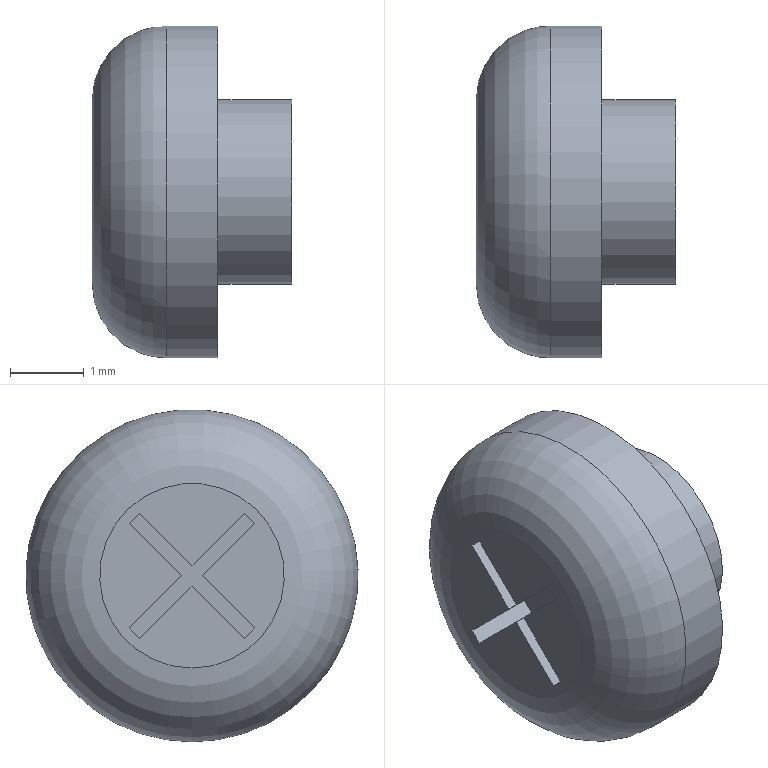Part | STEP file | 1 solid | 19 faces | box 2.7 x 4.5 x 4.5 mm | volume 28.373 mm3 | plane 16 | cylinder 2 | torus 1 | commonest cylinder face diameters 2.5 x1 4.5 x1
STEP:
#1=CARTESIAN_POINT('',(0.,0.,0.));
#2=DIRECTION('',(0.,0.,1.));
#3=DIRECTION('',(1.,0.,0.));
#4=AXIS2_PLACEMENT_3D('',#1,#2,#3);
#5=CARTESIAN_POINT('',(0.,0.,-1.25));
#6=VERTEX_POINT('',#5);
#7=CARTESIAN_POINT('',(0.,0.,0.));
#8=DIRECTION('',(-1.,0.,0.));
#9=DIRECTION('',(0.,0.,-1.));
#10=AXIS2_PLACEMENT_3D('',#7,#8,#9);
#11=CIRCLE('',#10,1.25);
#12=CARTESIAN_POINT('',(0.,0.,0.));
#13=DIRECTION('',(1.,0.,0.));
#14=DIRECTION('',(0.,0.,-1.));
#15=AXIS2_PLACEMENT_3D('',#12,#13,#14);
#16=PLANE('',#15);
#17=CARTESIAN_POINT('',(1.25,0.));
#18=CARTESIAN_POINT('',(1.25,-2.165));
#19=CARTESIAN_POINT('',(-0.625,-1.083));
#20=CARTESIAN_POINT('',(-2.5,0.));
#21=CARTESIAN_POINT('',(-0.625,1.083));
#22=CARTESIAN_POINT('',(1.25,2.165));
#23=CARTESIAN_POINT('',(1.25,0.));
#24=(BOUNDED_CURVE()B_SPLINE_CURVE(2,(#17,#18,#19,#20,#21,#22,#23),.UNSPECIFIED.,.T.,.F.)B_SPLINE_CURVE_WITH_KNOTS((1,2,2,2,2,1),(-2.094,0.,2.094,4.189,6.283,8.378),.UNSPECIFIED.)CURVE()GEOMETRIC_REPRESENTATION_ITEM()RATIONAL_B_SPLINE_CURVE((1.,0.5,1.,0.5,1.,0.5,1.))REPRESENTATION_ITEM(''));
#25=(GEOMETRIC_REPRESENTATION_CONTEXT(2)PARAMETRIC_REPRESENTATION_CONTEXT()REPRESENTATION_CONTEXT('',''));
#26=DEFINITIONAL_REPRESENTATION('',(#24),#25);
#27=PCURVE('',#16,#26);
#28=CARTESIAN_POINT('',(-1.835,0.,0.));
#29=DIRECTION('',(1.,0.,0.));
#30=DIRECTION('',(0.,0.,-1.));
#31=AXIS2_PLACEMENT_3D('',#28,#29,#30);
#32=CYLINDRICAL_SURFACE('',#31,1.25);
#33=CARTESIAN_POINT('',(6.283,1.835));
#34=DIRECTION('',(-1.,0.));
#35=VECTOR('',#34,1.);
#36=LINE('',#33,#35);
#37=(GEOMETRIC_REPRESENTATION_CONTEXT(2)PARAMETRIC_REPRESENTATION_CONTEXT()REPRESENTATION_CONTEXT('',''));
#38=DEFINITIONAL_REPRESENTATION('',(#36),#37);
#39=PCURVE('',#32,#38);
#40=SURFACE_CURVE('',#11,(#27,#39),.PCURVE_S1.);
#41=EDGE_CURVE('',#6,#6,#40,.T.);
#42=ORIENTED_EDGE('',*,*,#41,.T.);
#43=EDGE_LOOP('',(#42));
#44=FACE_BOUND('',#43,.T.);
#45=CARTESIAN_POINT('',(0.,0.,-2.25));
#46=VERTEX_POINT('',#45);
#47=CARTESIAN_POINT('',(0.,0.,0.));
#48=DIRECTION('',(1.,0.,0.));
#49=DIRECTION('',(0.,0.,-1.));
#50=AXIS2_PLACEMENT_3D('',#47,#48,#49);
#51=CIRCLE('',#50,2.25);
#52=CARTESIAN_POINT('',(0.,0.));
#53=DIRECTION('',(1.,0.));
#54=AXIS2_PLACEMENT_2D('',#52,#53);
#55=CIRCLE('',#54,2.25);
#56=(GEOMETRIC_REPRESENTATION_CONTEXT(2)PARAMETRIC_REPRESENTATION_CONTEXT()REPRESENTATION_CONTEXT('',''));
#57=DEFINITIONAL_REPRESENTATION('',(#55),#56);
#58=PCURVE('',#16,#57);
#59=CARTESIAN_POINT('',(-1.835,0.,0.));
#60=DIRECTION('',(1.,0.,0.));
#61=DIRECTION('',(0.,0.,-1.));
#62=AXIS2_PLACEMENT_3D('',#59,#60,#61);
#63=CYLINDRICAL_SURFACE('',#62,2.25);
#64=CARTESIAN_POINT('',(0.,1.835));
#65=DIRECTION('',(1.,0.));
#66=VECTOR('',#65,1.);
#67=LINE('',#64,#66);
#68=(GEOMETRIC_REPRESENTATION_CONTEXT(2)PARAMETRIC_REPRESENTATION_CONTEXT()REPRESENTATION_CONTEXT('',''));
#69=DEFINITIONAL_REPRESENTATION('',(#67),#68);
#70=PCURVE('',#63,#69);
#71=SURFACE_CURVE('',#51,(#58,#70),.PCURVE_S1.);
#72=EDGE_CURVE('',#46,#46,#71,.T.);
#73=ORIENTED_EDGE('',*,*,#72,.T.);
#74=EDGE_LOOP('',(#73));
#75=FACE_BOUND('',#74,.T.);
#76=ADVANCED_FACE('',(#44,#75),#16,.T.);
#77=CARTESIAN_POINT('',(1.,0.,-1.25));
#78=VERTEX_POINT('',#77);
#79=CARTESIAN_POINT('',(1.,0.,0.));
#80=DIRECTION('',(-1.,0.,0.));
#81=DIRECTION('',(0.,0.,-1.));
#82=AXIS2_PLACEMENT_3D('',#79,#80,#81);
#83=CIRCLE('',#82,1.25);
#84=CARTESIAN_POINT('',(6.283,2.835));
#85=DIRECTION('',(-1.,0.));
#86=VECTOR('',#85,1.);
#87=LINE('',#84,#86);
#88=(GEOMETRIC_REPRESENTATION_CONTEXT(2)PARAMETRIC_REPRESENTATION_CONTEXT()REPRESENTATION_CONTEXT('',''));
#89=DEFINITIONAL_REPRESENTATION('',(#87),#88);
#90=PCURVE('',#32,#89);
#91=CARTESIAN_POINT('',(1.,0.,0.));
#92=DIRECTION('',(1.,0.,0.));
#93=DIRECTION('',(0.,0.,-1.));
#94=AXIS2_PLACEMENT_3D('',#91,#92,#93);
#95=PLANE('',#94);
#96=CARTESIAN_POINT('',(1.25,0.));
#97=CARTESIAN_POINT('',(1.25,-2.165));
#98=CARTESIAN_POINT('',(-0.625,-1.083));
#99=CARTESIAN_POINT('',(-2.5,0.));
#100=CARTESIAN_POINT('',(-0.625,1.083));
#101=CARTESIAN_POINT('',(1.25,2.165));
#102=CARTESIAN_POINT('',(1.25,0.));
#103=(BOUNDED_CURVE()B_SPLINE_CURVE(2,(#96,#97,#98,#99,#100,#101,#102),.UNSPECIFIED.,.T.,.F.)B_SPLINE_CURVE_WITH_KNOTS((1,2,2,2,2,1),(-2.094,0.,2.094,4.189,6.283,8.378),.UNSPECIFIED.)CURVE()GEOMETRIC_REPRESENTATION_ITEM()RATIONAL_B_SPLINE_CURVE((1.,0.5,1.,0.5,1.,0.5,1.))REPRESENTATION_ITEM(''));
#104=(GEOMETRIC_REPRESENTATION_CONTEXT(2)PARAMETRIC_REPRESENTATION_CONTEXT()REPRESENTATION_CONTEXT('',''));
#105=DEFINITIONAL_REPRESENTATION('',(#103),#104);
#106=PCURVE('',#95,#105);
#107=SURFACE_CURVE('',#83,(#90,#106),.PCURVE_S1.);
#108=EDGE_CURVE('',#78,#78,#107,.T.);
#109=ORIENTED_EDGE('',*,*,#108,.T.);
#110=CARTESIAN_POINT('',(0.,0.,-1.25));
#111=CARTESIAN_POINT('',(1.,0.,-1.25));
#112=B_SPLINE_CURVE_WITH_KNOTS('',1,(#110,#111),.UNSPECIFIED.,.F.,.F.,(2,2),(1.835,2.835),.PIECEWISE_BEZIER_KNOTS.);
#113=CARTESIAN_POINT('',(0.,0.));
#114=DIRECTION('',(0.,1.));
#115=VECTOR('',#114,1.);
#116=LINE('',#113,#115);
#117=(GEOMETRIC_REPRESENTATION_CONTEXT(2)PARAMETRIC_REPRESENTATION_CONTEXT()REPRESENTATION_CONTEXT('',''));
#118=DEFINITIONAL_REPRESENTATION('',(#116),#117);
#119=PCURVE('',#32,#118);
#120=CARTESIAN_POINT('',(6.283,0.));
#121=DIRECTION('',(0.,1.));
#122=VECTOR('',#121,1.);
#123=LINE('',#120,#122);
#124=(GEOMETRIC_REPRESENTATION_CONTEXT(2)PARAMETRIC_REPRESENTATION_CONTEXT()REPRESENTATION_CONTEXT('',''));
#125=DEFINITIONAL_REPRESENTATION('',(#123),#124);
#126=PCURVE('',#32,#125);
#127=SEAM_CURVE('',#112,(#119,#126),.PCURVE_S1.);
#128=EDGE_CURVE('',#6,#78,#127,.T.);
#129=ORIENTED_EDGE('',*,*,#128,.F.);
#130=ORIENTED_EDGE('',*,*,#41,.F.);
#131=ORIENTED_EDGE('',*,*,#128,.T.);
#132=EDGE_LOOP('',(#109,#129,#130,#131));
#133=FACE_BOUND('',#132,.T.);
#134=ADVANCED_FACE('',(#133),#32,.T.);
#135=CARTESIAN_POINT('',(-0.7,0.,-2.25));
#136=VERTEX_POINT('',#135);
#137=CARTESIAN_POINT('',(-0.7,0.,0.));
#138=DIRECTION('',(1.,0.,0.));
#139=DIRECTION('',(0.,0.,-1.));
#140=AXIS2_PLACEMENT_3D('',#137,#138,#139);
#141=CIRCLE('',#140,2.25);
#142=CARTESIAN_POINT('',(0.,1.135));
#143=DIRECTION('',(1.,0.));
#144=VECTOR('',#143,1.);
#145=LINE('',#142,#144);
#146=(GEOMETRIC_REPRESENTATION_CONTEXT(2)PARAMETRIC_REPRESENTATION_CONTEXT()REPRESENTATION_CONTEXT('',''));
#147=DEFINITIONAL_REPRESENTATION('',(#145),#146);
#148=PCURVE('',#63,#147);
#149=CARTESIAN_POINT('',(-0.7,0.,0.));
#150=DIRECTION('',(1.,0.,0.));
#151=DIRECTION('',(0.,0.,-1.));
#152=AXIS2_PLACEMENT_3D('',#149,#150,#151);
#153=TOROIDAL_SURFACE('',#152,1.25,1.);
#154=CARTESIAN_POINT('',(0.,6.283));
#155=DIRECTION('',(1.,0.));
#156=VECTOR('',#155,1.);
#157=LINE('',#154,#156);
#158=(GEOMETRIC_REPRESENTATION_CONTEXT(2)PARAMETRIC_REPRESENTATION_CONTEXT()REPRESENTATION_CONTEXT('',''));
#159=DEFINITIONAL_REPRESENTATION('',(#157),#158);
#160=PCURVE('',#153,#159);
#161=SURFACE_CURVE('',#141,(#148,#160),.PCURVE_S1.);
#162=EDGE_CURVE('',#136,#136,#161,.T.);
#163=ORIENTED_EDGE('',*,*,#162,.T.);
#164=CARTESIAN_POINT('',(-0.7,0.,-2.25));
#165=CARTESIAN_POINT('',(0.,0.,-2.25));
#166=B_SPLINE_CURVE_WITH_KNOTS('',1,(#164,#165),.UNSPECIFIED.,.F.,.F.,(2,2),(1.135,1.835),.PIECEWISE_BEZIER_KNOTS.);
#167=CARTESIAN_POINT('',(6.283,0.));
#168=DIRECTION('',(0.,1.));
#169=VECTOR('',#168,1.);
#170=LINE('',#167,#169);
#171=(GEOMETRIC_REPRESENTATION_CONTEXT(2)PARAMETRIC_REPRESENTATION_CONTEXT()REPRESENTATION_CONTEXT('',''));
#172=DEFINITIONAL_REPRESENTATION('',(#170),#171);
#173=PCURVE('',#63,#172);
#174=CARTESIAN_POINT('',(0.,0.));
#175=DIRECTION('',(0.,1.));
#176=VECTOR('',#175,1.);
#177=LINE('',#174,#176);
#178=(GEOMETRIC_REPRESENTATION_CONTEXT(2)PARAMETRIC_REPRESENTATION_CONTEXT()REPRESENTATION_CONTEXT('',''));
#179=DEFINITIONAL_REPRESENTATION('',(#177),#178);
#180=PCURVE('',#63,#179);
#181=SEAM_CURVE('',#166,(#173,#180),.PCURVE_S1.);
#182=EDGE_CURVE('',#136,#46,#181,.T.);
#183=ORIENTED_EDGE('',*,*,#182,.T.);
#184=ORIENTED_EDGE('',*,*,#72,.F.);
#185=ORIENTED_EDGE('',*,*,#182,.F.);
#186=EDGE_LOOP('',(#163,#183,#184,#185));
#187=FACE_BOUND('',#186,.T.);
#188=ADVANCED_FACE('',(#187),#63,.T.);
#189=ORIENTED_EDGE('',*,*,#108,.F.);
#190=EDGE_LOOP('',(#189));
#191=FACE_BOUND('',#190,.T.);
#192=ADVANCED_FACE('',(#191),#95,.T.);
#193=ORIENTED_EDGE('',*,*,#162,.F.);
#194=CARTESIAN_POINT('',(-1.7,0.,-1.25));
#195=VERTEX_POINT('',#194);
#196=CARTESIAN_POINT('',(-1.7,0.,-1.25));
#197=CARTESIAN_POINT('',(-1.7,0.,-1.517));
#198=CARTESIAN_POINT('',(-1.615,0.,-1.778));
#199=CARTESIAN_POINT('',(-1.452,0.,-2.002));
#200=CARTESIAN_POINT('',(-1.228,0.,-2.165));
#201=CARTESIAN_POINT('',(-0.9673,0.,-2.25));
#202=CARTESIAN_POINT('',(-0.7,0.,-2.25));
#203=(BOUNDED_CURVE()B_SPLINE_CURVE(6,(#196,#197,#198,#199,#200,#201,#202),.UNSPECIFIED.,.F.,.F.)B_SPLINE_CURVE_WITH_KNOTS((7,7),(4.712,6.283),.PIECEWISE_BEZIER_KNOTS.)CURVE()GEOMETRIC_REPRESENTATION_ITEM()RATIONAL_B_SPLINE_CURVE((1.031,1.01,0.9979,0.994,0.9979,1.01,1.031))REPRESENTATION_ITEM(''));
#204=CARTESIAN_POINT('',(0.,0.));
#205=DIRECTION('',(0.,1.));
#206=VECTOR('',#205,1.);
#207=LINE('',#204,#206);
#208=(GEOMETRIC_REPRESENTATION_CONTEXT(2)PARAMETRIC_REPRESENTATION_CONTEXT()REPRESENTATION_CONTEXT('',''));
#209=DEFINITIONAL_REPRESENTATION('',(#207),#208);
#210=PCURVE('',#153,#209);
#211=CARTESIAN_POINT('',(6.283,0.));
#212=DIRECTION('',(0.,1.));
#213=VECTOR('',#212,1.);
#214=LINE('',#211,#213);
#215=(GEOMETRIC_REPRESENTATION_CONTEXT(2)PARAMETRIC_REPRESENTATION_CONTEXT()REPRESENTATION_CONTEXT('',''));
#216=DEFINITIONAL_REPRESENTATION('',(#214),#215);
#217=PCURVE('',#153,#216);
#218=SEAM_CURVE('',#203,(#210,#217),.PCURVE_S1.);
#219=EDGE_CURVE('',#195,#136,#218,.T.);
#220=ORIENTED_EDGE('',*,*,#219,.F.);
#221=CARTESIAN_POINT('',(-1.7,0.,0.));
#222=DIRECTION('',(1.,0.,0.));
#223=DIRECTION('',(0.,0.,-1.));
#224=AXIS2_PLACEMENT_3D('',#221,#222,#223);
#225=CIRCLE('',#224,1.25);
#226=CARTESIAN_POINT('',(0.,4.712));
#227=DIRECTION('',(1.,0.));
#228=VECTOR('',#227,1.);
#229=LINE('',#226,#228);
#230=(GEOMETRIC_REPRESENTATION_CONTEXT(2)PARAMETRIC_REPRESENTATION_CONTEXT()REPRESENTATION_CONTEXT('',''));
#231=DEFINITIONAL_REPRESENTATION('',(#229),#230);
#232=PCURVE('',#153,#231);
#233=CARTESIAN_POINT('',(-1.7,0.,0.));
#234=DIRECTION('',(1.,0.,0.));
#235=DIRECTION('',(0.,0.,-1.));
#236=AXIS2_PLACEMENT_3D('',#233,#234,#235);
#237=PLANE('',#236);
#238=CARTESIAN_POINT('',(0.,0.));
#239=DIRECTION('',(1.,0.));
#240=AXIS2_PLACEMENT_2D('',#238,#239);
#241=CIRCLE('',#240,1.25);
#242=(GEOMETRIC_REPRESENTATION_CONTEXT(2)PARAMETRIC_REPRESENTATION_CONTEXT()REPRESENTATION_CONTEXT('',''));
#243=DEFINITIONAL_REPRESENTATION('',(#241),#242);
#244=PCURVE('',#237,#243);
#245=SURFACE_CURVE('',#225,(#232,#244),.PCURVE_S1.);
#246=EDGE_CURVE('',#195,#195,#245,.T.);
#247=ORIENTED_EDGE('',*,*,#246,.T.);
#248=ORIENTED_EDGE('',*,*,#219,.T.);
#249=EDGE_LOOP('',(#193,#220,#247,#248));
#250=FACE_BOUND('',#249,.T.);
#251=ADVANCED_FACE('',(#250),#153,.T.);
#252=CARTESIAN_POINT('',(-1.7,0.8485,0.7071));
#253=VERTEX_POINT('',#252);
#254=CARTESIAN_POINT('',(-1.7,0.1414,0.));
#255=VERTEX_POINT('',#254);
#256=CARTESIAN_POINT('',(-1.7,0.8485,0.7071));
#257=DIRECTION('',(0.,-0.7071,-0.7071));
#258=VECTOR('',#257,1.);
#259=LINE('',#256,#258);
#260=CARTESIAN_POINT('',(-0.7071,0.8485));
#261=DIRECTION('',(0.7071,-0.7071));
#262=VECTOR('',#261,1.);
#263=LINE('',#260,#262);
#264=(GEOMETRIC_REPRESENTATION_CONTEXT(2)PARAMETRIC_REPRESENTATION_CONTEXT()REPRESENTATION_CONTEXT('',''));
#265=DEFINITIONAL_REPRESENTATION('',(#263),#264);
#266=PCURVE('',#237,#265);
#267=CARTESIAN_POINT('',(-1.7,0.8485,0.7071));
#268=DIRECTION('',(0.,0.7071,-0.7071));
#269=DIRECTION('',(0.,0.7071,0.7071));
#270=AXIS2_PLACEMENT_3D('',#267,#268,#269);
#271=PLANE('',#270);
#272=CARTESIAN_POINT('',(0.,0.));
#273=DIRECTION('',(-1.,0.));
#274=VECTOR('',#273,1.);
#275=LINE('',#272,#274);
#276=(GEOMETRIC_REPRESENTATION_CONTEXT(2)PARAMETRIC_REPRESENTATION_CONTEXT()REPRESENTATION_CONTEXT('',''));
#277=DEFINITIONAL_REPRESENTATION('',(#275),#276);
#278=PCURVE('',#271,#277);
#279=SURFACE_CURVE('',#259,(#266,#278),.PCURVE_S1.);
#280=EDGE_CURVE('',#253,#255,#279,.T.);
#281=ORIENTED_EDGE('',*,*,#280,.F.);
#282=CARTESIAN_POINT('',(-1.7,0.7071,0.8485));
#283=VERTEX_POINT('',#282);
#284=CARTESIAN_POINT('',(-1.7,0.7071,0.8485));
#285=DIRECTION('',(0.,0.7071,-0.7071));
#286=VECTOR('',#285,1.);
#287=LINE('',#284,#286);
#288=CARTESIAN_POINT('',(-0.8485,0.7071));
#289=DIRECTION('',(0.7071,0.7071));
#290=VECTOR('',#289,1.);
#291=LINE('',#288,#290);
#292=(GEOMETRIC_REPRESENTATION_CONTEXT(2)PARAMETRIC_REPRESENTATION_CONTEXT()REPRESENTATION_CONTEXT('',''));
#293=DEFINITIONAL_REPRESENTATION('',(#291),#292);
#294=PCURVE('',#237,#293);
#295=CARTESIAN_POINT('',(-1.7,0.7071,0.8485));
#296=DIRECTION('',(0.,0.7071,0.7071));
#297=DIRECTION('',(0.,-0.7071,0.7071));
#298=AXIS2_PLACEMENT_3D('',#295,#296,#297);
#299=PLANE('',#298);
#300=CARTESIAN_POINT('',(0.,0.));
#301=DIRECTION('',(-1.,0.));
#302=VECTOR('',#301,1.);
#303=LINE('',#300,#302);
#304=(GEOMETRIC_REPRESENTATION_CONTEXT(2)PARAMETRIC_REPRESENTATION_CONTEXT()REPRESENTATION_CONTEXT('',''));
#305=DEFINITIONAL_REPRESENTATION('',(#303),#304);
#306=PCURVE('',#299,#305);
#307=SURFACE_CURVE('',#287,(#294,#306),.PCURVE_S1.);
#308=EDGE_CURVE('',#283,#253,#307,.T.);
#309=ORIENTED_EDGE('',*,*,#308,.F.);
#310=CARTESIAN_POINT('',(-1.7,0.,0.1414));
#311=VERTEX_POINT('',#310);
#312=CARTESIAN_POINT('',(-1.7,0.,0.1414));
#313=DIRECTION('',(0.,0.7071,0.7071));
#314=VECTOR('',#313,1.);
#315=LINE('',#312,#314);
#316=CARTESIAN_POINT('',(-0.1414,0.));
#317=DIRECTION('',(-0.7071,0.7071));
#318=VECTOR('',#317,1.);
#319=LINE('',#316,#318);
#320=(GEOMETRIC_REPRESENTATION_CONTEXT(2)PARAMETRIC_REPRESENTATION_CONTEXT()REPRESENTATION_CONTEXT('',''));
#321=DEFINITIONAL_REPRESENTATION('',(#319),#320);
#322=PCURVE('',#237,#321);
#323=CARTESIAN_POINT('',(-1.7,0.,0.1414));
#324=DIRECTION('',(0.,-0.7071,0.7071));
#325=DIRECTION('',(0.,-0.7071,-0.7071));
#326=AXIS2_PLACEMENT_3D('',#323,#324,#325);
#327=PLANE('',#326);
#328=CARTESIAN_POINT('',(0.,0.));
#329=DIRECTION('',(-1.,0.));
#330=VECTOR('',#329,1.);
#331=LINE('',#328,#330);
#332=(GEOMETRIC_REPRESENTATION_CONTEXT(2)PARAMETRIC_REPRESENTATION_CONTEXT()REPRESENTATION_CONTEXT('',''));
#333=DEFINITIONAL_REPRESENTATION('',(#331),#332);
#334=PCURVE('',#327,#333);
#335=SURFACE_CURVE('',#315,(#322,#334),.PCURVE_S1.);
#336=EDGE_CURVE('',#311,#283,#335,.T.);
#337=ORIENTED_EDGE('',*,*,#336,.F.);
#338=CARTESIAN_POINT('',(-1.7,-0.7071,0.8485));
#339=VERTEX_POINT('',#338);
#340=CARTESIAN_POINT('',(-1.7,-0.7071,0.8485));
#341=DIRECTION('',(0.,0.7071,-0.7071));
#342=VECTOR('',#341,1.);
#343=LINE('',#340,#342);
#344=CARTESIAN_POINT('',(-0.8485,-0.7071));
#345=DIRECTION('',(0.7071,0.7071));
#346=VECTOR('',#345,1.);
#347=LINE('',#344,#346);
#348=(GEOMETRIC_REPRESENTATION_CONTEXT(2)PARAMETRIC_REPRESENTATION_CONTEXT()REPRESENTATION_CONTEXT('',''));
#349=DEFINITIONAL_REPRESENTATION('',(#347),#348);
#350=PCURVE('',#237,#349);
#351=CARTESIAN_POINT('',(-1.7,-0.7071,0.8485));
#352=DIRECTION('',(0.,0.7071,0.7071));
#353=DIRECTION('',(0.,-0.7071,0.7071));
#354=AXIS2_PLACEMENT_3D('',#351,#352,#353);
#355=PLANE('',#354);
#356=CARTESIAN_POINT('',(0.,0.));
#357=DIRECTION('',(-1.,0.));
#358=VECTOR('',#357,1.);
#359=LINE('',#356,#358);
#360=(GEOMETRIC_REPRESENTATION_CONTEXT(2)PARAMETRIC_REPRESENTATION_CONTEXT()REPRESENTATION_CONTEXT('',''));
#361=DEFINITIONAL_REPRESENTATION('',(#359),#360);
#362=PCURVE('',#355,#361);
#363=SURFACE_CURVE('',#343,(#350,#362),.PCURVE_S1.);
#364=EDGE_CURVE('',#339,#311,#363,.T.);
#365=ORIENTED_EDGE('',*,*,#364,.F.);
#366=CARTESIAN_POINT('',(-1.7,-0.8485,0.7071));
#367=VERTEX_POINT('',#366);
#368=CARTESIAN_POINT('',(-1.7,-0.8485,0.7071));
#369=DIRECTION('',(0.,0.7071,0.7071));
#370=VECTOR('',#369,1.);
#371=LINE('',#368,#370);
#372=CARTESIAN_POINT('',(-0.7071,-0.8485));
#373=DIRECTION('',(-0.7071,0.7071));
#374=VECTOR('',#373,1.);
#375=LINE('',#372,#374);
#376=(GEOMETRIC_REPRESENTATION_CONTEXT(2)PARAMETRIC_REPRESENTATION_CONTEXT()REPRESENTATION_CONTEXT('',''));
#377=DEFINITIONAL_REPRESENTATION('',(#375),#376);
#378=PCURVE('',#237,#377);
#379=CARTESIAN_POINT('',(-1.7,-0.8485,0.7071));
#380=DIRECTION('',(0.,-0.7071,0.7071));
#381=DIRECTION('',(0.,-0.7071,-0.7071));
#382=AXIS2_PLACEMENT_3D('',#379,#380,#381);
#383=PLANE('',#382);
#384=CARTESIAN_POINT('',(0.,0.));
#385=DIRECTION('',(-1.,0.));
#386=VECTOR('',#385,1.);
#387=LINE('',#384,#386);
#388=(GEOMETRIC_REPRESENTATION_CONTEXT(2)PARAMETRIC_REPRESENTATION_CONTEXT()REPRESENTATION_CONTEXT('',''));
#389=DEFINITIONAL_REPRESENTATION('',(#387),#388);
#390=PCURVE('',#383,#389);
#391=SURFACE_CURVE('',#371,(#378,#390),.PCURVE_S1.);
#392=EDGE_CURVE('',#367,#339,#391,.T.);
#393=ORIENTED_EDGE('',*,*,#392,.F.);
#394=CARTESIAN_POINT('',(-1.7,-0.1414,0.));
#395=VERTEX_POINT('',#394);
#396=CARTESIAN_POINT('',(-1.7,-0.1414,0.));
#397=DIRECTION('',(0.,-0.7071,0.7071));
#398=VECTOR('',#397,1.);
#399=LINE('',#396,#398);
#400=CARTESIAN_POINT('',(0.,-0.1414));
#401=DIRECTION('',(-0.7071,-0.7071));
#402=VECTOR('',#401,1.);
#403=LINE('',#400,#402);
#404=(GEOMETRIC_REPRESENTATION_CONTEXT(2)PARAMETRIC_REPRESENTATION_CONTEXT()REPRESENTATION_CONTEXT('',''));
#405=DEFINITIONAL_REPRESENTATION('',(#403),#404);
#406=PCURVE('',#237,#405);
#407=CARTESIAN_POINT('',(-1.7,-0.1414,0.));
#408=DIRECTION('',(0.,-0.7071,-0.7071));
#409=DIRECTION('',(0.,0.7071,-0.7071));
#410=AXIS2_PLACEMENT_3D('',#407,#408,#409);
#411=PLANE('',#410);
#412=CARTESIAN_POINT('',(0.,0.));
#413=DIRECTION('',(-1.,0.));
#414=VECTOR('',#413,1.);
#415=LINE('',#412,#414);
#416=(GEOMETRIC_REPRESENTATION_CONTEXT(2)PARAMETRIC_REPRESENTATION_CONTEXT()REPRESENTATION_CONTEXT('',''));
#417=DEFINITIONAL_REPRESENTATION('',(#415),#416);
#418=PCURVE('',#411,#417);
#419=SURFACE_CURVE('',#399,(#406,#418),.PCURVE_S1.);
#420=EDGE_CURVE('',#395,#367,#419,.T.);
#421=ORIENTED_EDGE('',*,*,#420,.F.);
#422=CARTESIAN_POINT('',(-1.7,-0.8485,-0.7071));
#423=VERTEX_POINT('',#422);
#424=CARTESIAN_POINT('',(-1.7,-0.8485,-0.7071));
#425=DIRECTION('',(0.,0.7071,0.7071));
#426=VECTOR('',#425,1.);
#427=LINE('',#424,#426);
#428=CARTESIAN_POINT('',(0.7071,-0.8485));
#429=DIRECTION('',(-0.7071,0.7071));
#430=VECTOR('',#429,1.);
#431=LINE('',#428,#430);
#432=(GEOMETRIC_REPRESENTATION_CONTEXT(2)PARAMETRIC_REPRESENTATION_CONTEXT()REPRESENTATION_CONTEXT('',''));
#433=DEFINITIONAL_REPRESENTATION('',(#431),#432);
#434=PCURVE('',#237,#433);
#435=CARTESIAN_POINT('',(-1.7,-0.8485,-0.7071));
#436=DIRECTION('',(0.,-0.7071,0.7071));
#437=DIRECTION('',(0.,-0.7071,-0.7071));
#438=AXIS2_PLACEMENT_3D('',#435,#436,#437);
#439=PLANE('',#438);
#440=CARTESIAN_POINT('',(0.,0.));
#441=DIRECTION('',(-1.,0.));
#442=VECTOR('',#441,1.);
#443=LINE('',#440,#442);
#444=(GEOMETRIC_REPRESENTATION_CONTEXT(2)PARAMETRIC_REPRESENTATION_CONTEXT()REPRESENTATION_CONTEXT('',''));
#445=DEFINITIONAL_REPRESENTATION('',(#443),#444);
#446=PCURVE('',#439,#445);
#447=SURFACE_CURVE('',#427,(#434,#446),.PCURVE_S1.);
#448=EDGE_CURVE('',#423,#395,#447,.T.);
#449=ORIENTED_EDGE('',*,*,#448,.F.);
#450=CARTESIAN_POINT('',(-1.7,-0.7071,-0.8485));
#451=VERTEX_POINT('',#450);
#452=CARTESIAN_POINT('',(-1.7,-0.7071,-0.8485));
#453=DIRECTION('',(0.,-0.7071,0.7071));
#454=VECTOR('',#453,1.);
#455=LINE('',#452,#454);
#456=CARTESIAN_POINT('',(0.8485,-0.7071));
#457=DIRECTION('',(-0.7071,-0.7071));
#458=VECTOR('',#457,1.);
#459=LINE('',#456,#458);
#460=(GEOMETRIC_REPRESENTATION_CONTEXT(2)PARAMETRIC_REPRESENTATION_CONTEXT()REPRESENTATION_CONTEXT('',''));
#461=DEFINITIONAL_REPRESENTATION('',(#459),#460);
#462=PCURVE('',#237,#461);
#463=CARTESIAN_POINT('',(-1.7,-0.7071,-0.8485));
#464=DIRECTION('',(0.,-0.7071,-0.7071));
#465=DIRECTION('',(0.,0.7071,-0.7071));
#466=AXIS2_PLACEMENT_3D('',#463,#464,#465);
#467=PLANE('',#466);
#468=CARTESIAN_POINT('',(0.,0.));
#469=DIRECTION('',(-1.,0.));
#470=VECTOR('',#469,1.);
#471=LINE('',#468,#470);
#472=(GEOMETRIC_REPRESENTATION_CONTEXT(2)PARAMETRIC_REPRESENTATION_CONTEXT()REPRESENTATION_CONTEXT('',''));
#473=DEFINITIONAL_REPRESENTATION('',(#471),#472);
#474=PCURVE('',#467,#473);
#475=SURFACE_CURVE('',#455,(#462,#474),.PCURVE_S1.);
#476=EDGE_CURVE('',#451,#423,#475,.T.);
#477=ORIENTED_EDGE('',*,*,#476,.F.);
#478=CARTESIAN_POINT('',(-1.7,0.,-0.1414));
#479=VERTEX_POINT('',#478);
#480=CARTESIAN_POINT('',(-1.7,0.,-0.1414));
#481=DIRECTION('',(0.,-0.7071,-0.7071));
#482=VECTOR('',#481,1.);
#483=LINE('',#480,#482);
#484=CARTESIAN_POINT('',(0.1414,0.));
#485=DIRECTION('',(0.7071,-0.7071));
#486=VECTOR('',#485,1.);
#487=LINE('',#484,#486);
#488=(GEOMETRIC_REPRESENTATION_CONTEXT(2)PARAMETRIC_REPRESENTATION_CONTEXT()REPRESENTATION_CONTEXT('',''));
#489=DEFINITIONAL_REPRESENTATION('',(#487),#488);
#490=PCURVE('',#237,#489);
#491=CARTESIAN_POINT('',(-1.7,0.,-0.1414));
#492=DIRECTION('',(0.,0.7071,-0.7071));
#493=DIRECTION('',(0.,0.7071,0.7071));
#494=AXIS2_PLACEMENT_3D('',#491,#492,#493);
#495=PLANE('',#494);
#496=CARTESIAN_POINT('',(0.,0.));
#497=DIRECTION('',(-1.,0.));
#498=VECTOR('',#497,1.);
#499=LINE('',#496,#498);
#500=(GEOMETRIC_REPRESENTATION_CONTEXT(2)PARAMETRIC_REPRESENTATION_CONTEXT()REPRESENTATION_CONTEXT('',''));
#501=DEFINITIONAL_REPRESENTATION('',(#499),#500);
#502=PCURVE('',#495,#501);
#503=SURFACE_CURVE('',#483,(#490,#502),.PCURVE_S1.);
#504=EDGE_CURVE('',#479,#451,#503,.T.);
#505=ORIENTED_EDGE('',*,*,#504,.F.);
#506=CARTESIAN_POINT('',(-1.7,0.7071,-0.8485));
#507=VERTEX_POINT('',#506);
#508=CARTESIAN_POINT('',(-1.7,0.7071,-0.8485));
#509=DIRECTION('',(0.,-0.7071,0.7071));
#510=VECTOR('',#509,1.);
#511=LINE('',#508,#510);
#512=CARTESIAN_POINT('',(0.8485,0.7071));
#513=DIRECTION('',(-0.7071,-0.7071));
#514=VECTOR('',#513,1.);
#515=LINE('',#512,#514);
#516=(GEOMETRIC_REPRESENTATION_CONTEXT(2)PARAMETRIC_REPRESENTATION_CONTEXT()REPRESENTATION_CONTEXT('',''));
#517=DEFINITIONAL_REPRESENTATION('',(#515),#516);
#518=PCURVE('',#237,#517);
#519=CARTESIAN_POINT('',(-1.7,0.7071,-0.8485));
#520=DIRECTION('',(0.,-0.7071,-0.7071));
#521=DIRECTION('',(0.,0.7071,-0.7071));
#522=AXIS2_PLACEMENT_3D('',#519,#520,#521);
#523=PLANE('',#522);
#524=CARTESIAN_POINT('',(0.,0.));
#525=DIRECTION('',(-1.,0.));
#526=VECTOR('',#525,1.);
#527=LINE('',#524,#526);
#528=(GEOMETRIC_REPRESENTATION_CONTEXT(2)PARAMETRIC_REPRESENTATION_CONTEXT()REPRESENTATION_CONTEXT('',''));
#529=DEFINITIONAL_REPRESENTATION('',(#527),#528);
#530=PCURVE('',#523,#529);
#531=SURFACE_CURVE('',#511,(#518,#530),.PCURVE_S1.);
#532=EDGE_CURVE('',#507,#479,#531,.T.);
#533=ORIENTED_EDGE('',*,*,#532,.F.);
#534=CARTESIAN_POINT('',(-1.7,0.8485,-0.7071));
#535=VERTEX_POINT('',#534);
#536=CARTESIAN_POINT('',(-1.7,0.8485,-0.7071));
#537=DIRECTION('',(0.,-0.7071,-0.7071));
#538=VECTOR('',#537,1.);
#539=LINE('',#536,#538);
#540=CARTESIAN_POINT('',(0.7071,0.8485));
#541=DIRECTION('',(0.7071,-0.7071));
#542=VECTOR('',#541,1.);
#543=LINE('',#540,#542);
#544=(GEOMETRIC_REPRESENTATION_CONTEXT(2)PARAMETRIC_REPRESENTATION_CONTEXT()REPRESENTATION_CONTEXT('',''));
#545=DEFINITIONAL_REPRESENTATION('',(#543),#544);
#546=PCURVE('',#237,#545);
#547=CARTESIAN_POINT('',(-1.7,0.8485,-0.7071));
#548=DIRECTION('',(0.,0.7071,-0.7071));
#549=DIRECTION('',(0.,0.7071,0.7071));
#550=AXIS2_PLACEMENT_3D('',#547,#548,#549);
#551=PLANE('',#550);
#552=CARTESIAN_POINT('',(0.,0.));
#553=DIRECTION('',(-1.,0.));
#554=VECTOR('',#553,1.);
#555=LINE('',#552,#554);
#556=(GEOMETRIC_REPRESENTATION_CONTEXT(2)PARAMETRIC_REPRESENTATION_CONTEXT()REPRESENTATION_CONTEXT('',''));
#557=DEFINITIONAL_REPRESENTATION('',(#555),#556);
#558=PCURVE('',#551,#557);
#559=SURFACE_CURVE('',#539,(#546,#558),.PCURVE_S1.);
#560=EDGE_CURVE('',#535,#507,#559,.T.);
#561=ORIENTED_EDGE('',*,*,#560,.F.);
#562=CARTESIAN_POINT('',(-1.7,0.1414,0.));
#563=DIRECTION('',(0.,0.7071,-0.7071));
#564=VECTOR('',#563,1.);
#565=LINE('',#562,#564);
#566=CARTESIAN_POINT('',(0.,0.1414));
#567=DIRECTION('',(0.7071,0.7071));
#568=VECTOR('',#567,1.);
#569=LINE('',#566,#568);
#570=(GEOMETRIC_REPRESENTATION_CONTEXT(2)PARAMETRIC_REPRESENTATION_CONTEXT()REPRESENTATION_CONTEXT('',''));
#571=DEFINITIONAL_REPRESENTATION('',(#569),#570);
#572=PCURVE('',#237,#571);
#573=CARTESIAN_POINT('',(-1.7,0.1414,0.));
#574=DIRECTION('',(0.,0.7071,0.7071));
#575=DIRECTION('',(0.,-0.7071,0.7071));
#576=AXIS2_PLACEMENT_3D('',#573,#574,#575);
#577=PLANE('',#576);
#578=CARTESIAN_POINT('',(0.,0.));
#579=DIRECTION('',(-1.,0.));
#580=VECTOR('',#579,1.);
#581=LINE('',#578,#580);
#582=(GEOMETRIC_REPRESENTATION_CONTEXT(2)PARAMETRIC_REPRESENTATION_CONTEXT()REPRESENTATION_CONTEXT('',''));
#583=DEFINITIONAL_REPRESENTATION('',(#581),#582);
#584=PCURVE('',#577,#583);
#585=SURFACE_CURVE('',#565,(#572,#584),.PCURVE_S1.);
#586=EDGE_CURVE('',#255,#535,#585,.T.);
#587=ORIENTED_EDGE('',*,*,#586,.F.);
#588=EDGE_LOOP('',(#281,#309,#337,#365,#393,#421,#449,#477,#505,#533,#561,#587));
#589=FACE_BOUND('',#588,.T.);
#590=ORIENTED_EDGE('',*,*,#246,.F.);
#591=EDGE_LOOP('',(#590));
#592=FACE_BOUND('',#591,.T.);
#593=ADVANCED_FACE('',(#589,#592),#237,.F.);
#594=CARTESIAN_POINT('',(-0.7,0.1414,0.));
#595=VERTEX_POINT('',#594);
#596=CARTESIAN_POINT('',(-1.7,0.1414,0.));
#597=DIRECTION('',(1.,0.,0.));
#598=VECTOR('',#597,1.);
#599=LINE('',#596,#598);
#600=CARTESIAN_POINT('',(0.,0.));
#601=DIRECTION('',(0.,1.));
#602=VECTOR('',#601,1.);
#603=LINE('',#600,#602);
#604=(GEOMETRIC_REPRESENTATION_CONTEXT(2)PARAMETRIC_REPRESENTATION_CONTEXT()REPRESENTATION_CONTEXT('',''));
#605=DEFINITIONAL_REPRESENTATION('',(#603),#604);
#606=PCURVE('',#577,#605);
#607=CARTESIAN_POINT('',(-1.,0.));
#608=DIRECTION('',(0.,1.));
#609=VECTOR('',#608,1.);
#610=LINE('',#607,#609);
#611=(GEOMETRIC_REPRESENTATION_CONTEXT(2)PARAMETRIC_REPRESENTATION_CONTEXT()REPRESENTATION_CONTEXT('',''));
#612=DEFINITIONAL_REPRESENTATION('',(#610),#611);
#613=PCURVE('',#271,#612);
#614=SURFACE_CURVE('',#599,(#606,#613),.PCURVE_S1.);
#615=EDGE_CURVE('',#255,#595,#614,.T.);
#616=ORIENTED_EDGE('',*,*,#615,.F.);
#617=ORIENTED_EDGE('',*,*,#586,.T.);
#618=CARTESIAN_POINT('',(-0.7,0.8485,-0.7071));
#619=VERTEX_POINT('',#618);
#620=CARTESIAN_POINT('',(-1.7,0.8485,-0.7071));
#621=DIRECTION('',(-1.,0.,0.));
#622=VECTOR('',#621,1.);
#623=LINE('',#620,#622);
#624=CARTESIAN_POINT('',(-1.,0.));
#625=DIRECTION('',(0.,-1.));
#626=VECTOR('',#625,1.);
#627=LINE('',#624,#626);
#628=(GEOMETRIC_REPRESENTATION_CONTEXT(2)PARAMETRIC_REPRESENTATION_CONTEXT()REPRESENTATION_CONTEXT('',''));
#629=DEFINITIONAL_REPRESENTATION('',(#627),#628);
#630=PCURVE('',#577,#629);
#631=CARTESIAN_POINT('',(0.,0.));
#632=DIRECTION('',(0.,-1.));
#633=VECTOR('',#632,1.);
#634=LINE('',#631,#633);
#635=(GEOMETRIC_REPRESENTATION_CONTEXT(2)PARAMETRIC_REPRESENTATION_CONTEXT()REPRESENTATION_CONTEXT('',''));
#636=DEFINITIONAL_REPRESENTATION('',(#634),#635);
#637=PCURVE('',#551,#636);
#638=SURFACE_CURVE('',#623,(#630,#637),.PCURVE_S1.);
#639=EDGE_CURVE('',#619,#535,#638,.T.);
#640=ORIENTED_EDGE('',*,*,#639,.F.);
#641=CARTESIAN_POINT('',(-0.7,0.1414,0.));
#642=DIRECTION('',(0.,0.7071,-0.7071));
#643=VECTOR('',#642,1.);
#644=LINE('',#641,#643);
#645=CARTESIAN_POINT('',(0.,1.));
#646=DIRECTION('',(-1.,0.));
#647=VECTOR('',#646,1.);
#648=LINE('',#645,#647);
#649=(GEOMETRIC_REPRESENTATION_CONTEXT(2)PARAMETRIC_REPRESENTATION_CONTEXT()REPRESENTATION_CONTEXT('',''));
#650=DEFINITIONAL_REPRESENTATION('',(#648),#649);
#651=PCURVE('',#577,#650);
#652=CARTESIAN_POINT('',(-0.7,0.,0.));
#653=DIRECTION('',(-1.,0.,0.));
#654=DIRECTION('',(0.,0.,1.));
#655=AXIS2_PLACEMENT_3D('',#652,#653,#654);
#656=PLANE('',#655);
#657=CARTESIAN_POINT('',(0.,0.1414));
#658=DIRECTION('',(-0.7071,0.7071));
#659=VECTOR('',#658,1.);
#660=LINE('',#657,#659);
#661=(GEOMETRIC_REPRESENTATION_CONTEXT(2)PARAMETRIC_REPRESENTATION_CONTEXT()REPRESENTATION_CONTEXT('',''));
#662=DEFINITIONAL_REPRESENTATION('',(#660),#661);
#663=PCURVE('',#656,#662);
#664=SURFACE_CURVE('',#644,(#651,#663),.PCURVE_S1.);
#665=EDGE_CURVE('',#595,#619,#664,.T.);
#666=ORIENTED_EDGE('',*,*,#665,.F.);
#667=EDGE_LOOP('',(#616,#617,#640,#666));
#668=FACE_BOUND('',#667,.T.);
#669=ADVANCED_FACE('',(#668),#577,.F.);
#670=CARTESIAN_POINT('',(-0.7,0.8485,0.7071));
#671=VERTEX_POINT('',#670);
#672=CARTESIAN_POINT('',(-1.7,0.8485,0.7071));
#673=DIRECTION('',(1.,0.,0.));
#674=VECTOR('',#673,1.);
#675=LINE('',#672,#674);
#676=CARTESIAN_POINT('',(0.,0.));
#677=DIRECTION('',(0.,1.));
#678=VECTOR('',#677,1.);
#679=LINE('',#676,#678);
#680=(GEOMETRIC_REPRESENTATION_CONTEXT(2)PARAMETRIC_REPRESENTATION_CONTEXT()REPRESENTATION_CONTEXT('',''));
#681=DEFINITIONAL_REPRESENTATION('',(#679),#680);
#682=PCURVE('',#271,#681);
#683=CARTESIAN_POINT('',(-0.2,0.));
#684=DIRECTION('',(0.,1.));
#685=VECTOR('',#684,1.);
#686=LINE('',#683,#685);
#687=(GEOMETRIC_REPRESENTATION_CONTEXT(2)PARAMETRIC_REPRESENTATION_CONTEXT()REPRESENTATION_CONTEXT('',''));
#688=DEFINITIONAL_REPRESENTATION('',(#686),#687);
#689=PCURVE('',#299,#688);
#690=SURFACE_CURVE('',#675,(#682,#689),.PCURVE_S1.);
#691=EDGE_CURVE('',#253,#671,#690,.T.);
#692=ORIENTED_EDGE('',*,*,#691,.F.);
#693=ORIENTED_EDGE('',*,*,#280,.T.);
#694=ORIENTED_EDGE('',*,*,#615,.T.);
#695=CARTESIAN_POINT('',(-0.7,0.8485,0.7071));
#696=DIRECTION('',(0.,-0.7071,-0.7071));
#697=VECTOR('',#696,1.);
#698=LINE('',#695,#697);
#699=CARTESIAN_POINT('',(0.,1.));
#700=DIRECTION('',(-1.,0.));
#701=VECTOR('',#700,1.);
#702=LINE('',#699,#701);
#703=(GEOMETRIC_REPRESENTATION_CONTEXT(2)PARAMETRIC_REPRESENTATION_CONTEXT()REPRESENTATION_CONTEXT('',''));
#704=DEFINITIONAL_REPRESENTATION('',(#702),#703);
#705=PCURVE('',#271,#704);
#706=CARTESIAN_POINT('',(0.7071,0.8485));
#707=DIRECTION('',(-0.7071,-0.7071));
#708=VECTOR('',#707,1.);
#709=LINE('',#706,#708);
#710=(GEOMETRIC_REPRESENTATION_CONTEXT(2)PARAMETRIC_REPRESENTATION_CONTEXT()REPRESENTATION_CONTEXT('',''));
#711=DEFINITIONAL_REPRESENTATION('',(#709),#710);
#712=PCURVE('',#656,#711);
#713=SURFACE_CURVE('',#698,(#705,#712),.PCURVE_S1.);
#714=EDGE_CURVE('',#671,#595,#713,.T.);
#715=ORIENTED_EDGE('',*,*,#714,.F.);
#716=EDGE_LOOP('',(#692,#693,#694,#715));
#717=FACE_BOUND('',#716,.T.);
#718=ADVANCED_FACE('',(#717),#271,.F.);
#719=CARTESIAN_POINT('',(-0.7,0.7071,0.8485));
#720=VERTEX_POINT('',#719);
#721=CARTESIAN_POINT('',(-1.7,0.7071,0.8485));
#722=DIRECTION('',(1.,0.,0.));
#723=VECTOR('',#722,1.);
#724=LINE('',#721,#723);
#725=CARTESIAN_POINT('',(0.,0.));
#726=DIRECTION('',(0.,1.));
#727=VECTOR('',#726,1.);
#728=LINE('',#725,#727);
#729=(GEOMETRIC_REPRESENTATION_CONTEXT(2)PARAMETRIC_REPRESENTATION_CONTEXT()REPRESENTATION_CONTEXT('',''));
#730=DEFINITIONAL_REPRESENTATION('',(#728),#729);
#731=PCURVE('',#299,#730);
#732=CARTESIAN_POINT('',(-1.,0.));
#733=DIRECTION('',(0.,1.));
#734=VECTOR('',#733,1.);
#735=LINE('',#732,#734);
#736=(GEOMETRIC_REPRESENTATION_CONTEXT(2)PARAMETRIC_REPRESENTATION_CONTEXT()REPRESENTATION_CONTEXT('',''));
#737=DEFINITIONAL_REPRESENTATION('',(#735),#736);
#738=PCURVE('',#327,#737);
#739=SURFACE_CURVE('',#724,(#731,#738),.PCURVE_S1.);
#740=EDGE_CURVE('',#283,#720,#739,.T.);
#741=ORIENTED_EDGE('',*,*,#740,.F.);
#742=ORIENTED_EDGE('',*,*,#308,.T.);
#743=ORIENTED_EDGE('',*,*,#691,.T.);
#744=CARTESIAN_POINT('',(-0.7,0.7071,0.8485));
#745=DIRECTION('',(0.,0.7071,-0.7071));
#746=VECTOR('',#745,1.);
#747=LINE('',#744,#746);
#748=CARTESIAN_POINT('',(0.,1.));
#749=DIRECTION('',(-1.,0.));
#750=VECTOR('',#749,1.);
#751=LINE('',#748,#750);
#752=(GEOMETRIC_REPRESENTATION_CONTEXT(2)PARAMETRIC_REPRESENTATION_CONTEXT()REPRESENTATION_CONTEXT('',''));
#753=DEFINITIONAL_REPRESENTATION('',(#751),#752);
#754=PCURVE('',#299,#753);
#755=CARTESIAN_POINT('',(0.8485,0.7071));
#756=DIRECTION('',(-0.7071,0.7071));
#757=VECTOR('',#756,1.);
#758=LINE('',#755,#757);
#759=(GEOMETRIC_REPRESENTATION_CONTEXT(2)PARAMETRIC_REPRESENTATION_CONTEXT()REPRESENTATION_CONTEXT('',''));
#760=DEFINITIONAL_REPRESENTATION('',(#758),#759);
#761=PCURVE('',#656,#760);
#762=SURFACE_CURVE('',#747,(#754,#761),.PCURVE_S1.);
#763=EDGE_CURVE('',#720,#671,#762,.T.);
#764=ORIENTED_EDGE('',*,*,#763,.F.);
#765=EDGE_LOOP('',(#741,#742,#743,#764));
#766=FACE_BOUND('',#765,.T.);
#767=ADVANCED_FACE('',(#766),#299,.F.);
#768=CARTESIAN_POINT('',(-0.7,0.,0.1414));
#769=VERTEX_POINT('',#768);
#770=CARTESIAN_POINT('',(-1.7,0.,0.1414));
#771=DIRECTION('',(1.,0.,0.));
#772=VECTOR('',#771,1.);
#773=LINE('',#770,#772);
#774=CARTESIAN_POINT('',(0.,0.));
#775=DIRECTION('',(0.,1.));
#776=VECTOR('',#775,1.);
#777=LINE('',#774,#776);
#778=(GEOMETRIC_REPRESENTATION_CONTEXT(2)PARAMETRIC_REPRESENTATION_CONTEXT()REPRESENTATION_CONTEXT('',''));
#779=DEFINITIONAL_REPRESENTATION('',(#777),#778);
#780=PCURVE('',#327,#779);
#781=CARTESIAN_POINT('',(-1.,0.));
#782=DIRECTION('',(0.,1.));
#783=VECTOR('',#782,1.);
#784=LINE('',#781,#783);
#785=(GEOMETRIC_REPRESENTATION_CONTEXT(2)PARAMETRIC_REPRESENTATION_CONTEXT()REPRESENTATION_CONTEXT('',''));
#786=DEFINITIONAL_REPRESENTATION('',(#784),#785);
#787=PCURVE('',#355,#786);
#788=SURFACE_CURVE('',#773,(#780,#787),.PCURVE_S1.);
#789=EDGE_CURVE('',#311,#769,#788,.T.);
#790=ORIENTED_EDGE('',*,*,#789,.F.);
#791=ORIENTED_EDGE('',*,*,#336,.T.);
#792=ORIENTED_EDGE('',*,*,#740,.T.);
#793=CARTESIAN_POINT('',(-0.7,0.,0.1414));
#794=DIRECTION('',(0.,0.7071,0.7071));
#795=VECTOR('',#794,1.);
#796=LINE('',#793,#795);
#797=CARTESIAN_POINT('',(0.,1.));
#798=DIRECTION('',(-1.,0.));
#799=VECTOR('',#798,1.);
#800=LINE('',#797,#799);
#801=(GEOMETRIC_REPRESENTATION_CONTEXT(2)PARAMETRIC_REPRESENTATION_CONTEXT()REPRESENTATION_CONTEXT('',''));
#802=DEFINITIONAL_REPRESENTATION('',(#800),#801);
#803=PCURVE('',#327,#802);
#804=CARTESIAN_POINT('',(0.1414,0.));
#805=DIRECTION('',(0.7071,0.7071));
#806=VECTOR('',#805,1.);
#807=LINE('',#804,#806);
#808=(GEOMETRIC_REPRESENTATION_CONTEXT(2)PARAMETRIC_REPRESENTATION_CONTEXT()REPRESENTATION_CONTEXT('',''));
#809=DEFINITIONAL_REPRESENTATION('',(#807),#808);
#810=PCURVE('',#656,#809);
#811=SURFACE_CURVE('',#796,(#803,#810),.PCURVE_S1.);
#812=EDGE_CURVE('',#769,#720,#811,.T.);
#813=ORIENTED_EDGE('',*,*,#812,.F.);
#814=EDGE_LOOP('',(#790,#791,#792,#813));
#815=FACE_BOUND('',#814,.T.);
#816=ADVANCED_FACE('',(#815),#327,.F.);
#817=CARTESIAN_POINT('',(-0.7,-0.7071,0.8485));
#818=VERTEX_POINT('',#817);
#819=CARTESIAN_POINT('',(-1.7,-0.7071,0.8485));
#820=DIRECTION('',(1.,0.,0.));
#821=VECTOR('',#820,1.);
#822=LINE('',#819,#821);
#823=CARTESIAN_POINT('',(0.,0.));
#824=DIRECTION('',(0.,1.));
#825=VECTOR('',#824,1.);
#826=LINE('',#823,#825);
#827=(GEOMETRIC_REPRESENTATION_CONTEXT(2)PARAMETRIC_REPRESENTATION_CONTEXT()REPRESENTATION_CONTEXT('',''));
#828=DEFINITIONAL_REPRESENTATION('',(#826),#827);
#829=PCURVE('',#355,#828);
#830=CARTESIAN_POINT('',(-0.2,0.));
#831=DIRECTION('',(0.,1.));
#832=VECTOR('',#831,1.);
#833=LINE('',#830,#832);
#834=(GEOMETRIC_REPRESENTATION_CONTEXT(2)PARAMETRIC_REPRESENTATION_CONTEXT()REPRESENTATION_CONTEXT('',''));
#835=DEFINITIONAL_REPRESENTATION('',(#833),#834);
#836=PCURVE('',#383,#835);
#837=SURFACE_CURVE('',#822,(#829,#836),.PCURVE_S1.);
#838=EDGE_CURVE('',#339,#818,#837,.T.);
#839=ORIENTED_EDGE('',*,*,#838,.F.);
#840=ORIENTED_EDGE('',*,*,#364,.T.);
#841=ORIENTED_EDGE('',*,*,#789,.T.);
#842=CARTESIAN_POINT('',(-0.7,-0.7071,0.8485));
#843=DIRECTION('',(0.,0.7071,-0.7071));
#844=VECTOR('',#843,1.);
#845=LINE('',#842,#844);
#846=CARTESIAN_POINT('',(0.,1.));
#847=DIRECTION('',(-1.,0.));
#848=VECTOR('',#847,1.);
#849=LINE('',#846,#848);
#850=(GEOMETRIC_REPRESENTATION_CONTEXT(2)PARAMETRIC_REPRESENTATION_CONTEXT()REPRESENTATION_CONTEXT('',''));
#851=DEFINITIONAL_REPRESENTATION('',(#849),#850);
#852=PCURVE('',#355,#851);
#853=CARTESIAN_POINT('',(0.8485,-0.7071));
#854=DIRECTION('',(-0.7071,0.7071));
#855=VECTOR('',#854,1.);
#856=LINE('',#853,#855);
#857=(GEOMETRIC_REPRESENTATION_CONTEXT(2)PARAMETRIC_REPRESENTATION_CONTEXT()REPRESENTATION_CONTEXT('',''));
#858=DEFINITIONAL_REPRESENTATION('',(#856),#857);
#859=PCURVE('',#656,#858);
#860=SURFACE_CURVE('',#845,(#852,#859),.PCURVE_S1.);
#861=EDGE_CURVE('',#818,#769,#860,.T.);
#862=ORIENTED_EDGE('',*,*,#861,.F.);
#863=EDGE_LOOP('',(#839,#840,#841,#862));
#864=FACE_BOUND('',#863,.T.);
#865=ADVANCED_FACE('',(#864),#355,.F.);
#866=CARTESIAN_POINT('',(-0.7,-0.8485,0.7071));
#867=VERTEX_POINT('',#866);
#868=CARTESIAN_POINT('',(-1.7,-0.8485,0.7071));
#869=DIRECTION('',(1.,0.,0.));
#870=VECTOR('',#869,1.);
#871=LINE('',#868,#870);
#872=CARTESIAN_POINT('',(0.,0.));
#873=DIRECTION('',(0.,1.));
#874=VECTOR('',#873,1.);
#875=LINE('',#872,#874);
#876=(GEOMETRIC_REPRESENTATION_CONTEXT(2)PARAMETRIC_REPRESENTATION_CONTEXT()REPRESENTATION_CONTEXT('',''));
#877=DEFINITIONAL_REPRESENTATION('',(#875),#876);
#878=PCURVE('',#383,#877);
#879=CARTESIAN_POINT('',(-1.,0.));
#880=DIRECTION('',(0.,1.));
#881=VECTOR('',#880,1.);
#882=LINE('',#879,#881);
#883=(GEOMETRIC_REPRESENTATION_CONTEXT(2)PARAMETRIC_REPRESENTATION_CONTEXT()REPRESENTATION_CONTEXT('',''));
#884=DEFINITIONAL_REPRESENTATION('',(#882),#883);
#885=PCURVE('',#411,#884);
#886=SURFACE_CURVE('',#871,(#878,#885),.PCURVE_S1.);
#887=EDGE_CURVE('',#367,#867,#886,.T.);
#888=ORIENTED_EDGE('',*,*,#887,.F.);
#889=ORIENTED_EDGE('',*,*,#392,.T.);
#890=ORIENTED_EDGE('',*,*,#838,.T.);
#891=CARTESIAN_POINT('',(-0.7,-0.8485,0.7071));
#892=DIRECTION('',(0.,0.7071,0.7071));
#893=VECTOR('',#892,1.);
#894=LINE('',#891,#893);
#895=CARTESIAN_POINT('',(0.,1.));
#896=DIRECTION('',(-1.,0.));
#897=VECTOR('',#896,1.);
#898=LINE('',#895,#897);
#899=(GEOMETRIC_REPRESENTATION_CONTEXT(2)PARAMETRIC_REPRESENTATION_CONTEXT()REPRESENTATION_CONTEXT('',''));
#900=DEFINITIONAL_REPRESENTATION('',(#898),#899);
#901=PCURVE('',#383,#900);
#902=CARTESIAN_POINT('',(0.7071,-0.8485));
#903=DIRECTION('',(0.7071,0.7071));
#904=VECTOR('',#903,1.);
#905=LINE('',#902,#904);
#906=(GEOMETRIC_REPRESENTATION_CONTEXT(2)PARAMETRIC_REPRESENTATION_CONTEXT()REPRESENTATION_CONTEXT('',''));
#907=DEFINITIONAL_REPRESENTATION('',(#905),#906);
#908=PCURVE('',#656,#907);
#909=SURFACE_CURVE('',#894,(#901,#908),.PCURVE_S1.);
#910=EDGE_CURVE('',#867,#818,#909,.T.);
#911=ORIENTED_EDGE('',*,*,#910,.F.);
#912=EDGE_LOOP('',(#888,#889,#890,#911));
#913=FACE_BOUND('',#912,.T.);
#914=ADVANCED_FACE('',(#913),#383,.F.);
#915=CARTESIAN_POINT('',(-0.7,-0.1414,0.));
#916=VERTEX_POINT('',#915);
#917=CARTESIAN_POINT('',(-1.7,-0.1414,0.));
#918=DIRECTION('',(1.,0.,0.));
#919=VECTOR('',#918,1.);
#920=LINE('',#917,#919);
#921=CARTESIAN_POINT('',(0.,0.));
#922=DIRECTION('',(0.,1.));
#923=VECTOR('',#922,1.);
#924=LINE('',#921,#923);
#925=(GEOMETRIC_REPRESENTATION_CONTEXT(2)PARAMETRIC_REPRESENTATION_CONTEXT()REPRESENTATION_CONTEXT('',''));
#926=DEFINITIONAL_REPRESENTATION('',(#924),#925);
#927=PCURVE('',#411,#926);
#928=CARTESIAN_POINT('',(-1.,0.));
#929=DIRECTION('',(0.,1.));
#930=VECTOR('',#929,1.);
#931=LINE('',#928,#930);
#932=(GEOMETRIC_REPRESENTATION_CONTEXT(2)PARAMETRIC_REPRESENTATION_CONTEXT()REPRESENTATION_CONTEXT('',''));
#933=DEFINITIONAL_REPRESENTATION('',(#931),#932);
#934=PCURVE('',#439,#933);
#935=SURFACE_CURVE('',#920,(#927,#934),.PCURVE_S1.);
#936=EDGE_CURVE('',#395,#916,#935,.T.);
#937=ORIENTED_EDGE('',*,*,#936,.F.);
#938=ORIENTED_EDGE('',*,*,#420,.T.);
#939=ORIENTED_EDGE('',*,*,#887,.T.);
#940=CARTESIAN_POINT('',(-0.7,-0.1414,0.));
#941=DIRECTION('',(0.,-0.7071,0.7071));
#942=VECTOR('',#941,1.);
#943=LINE('',#940,#942);
#944=CARTESIAN_POINT('',(0.,1.));
#945=DIRECTION('',(-1.,0.));
#946=VECTOR('',#945,1.);
#947=LINE('',#944,#946);
#948=(GEOMETRIC_REPRESENTATION_CONTEXT(2)PARAMETRIC_REPRESENTATION_CONTEXT()REPRESENTATION_CONTEXT('',''));
#949=DEFINITIONAL_REPRESENTATION('',(#947),#948);
#950=PCURVE('',#411,#949);
#951=CARTESIAN_POINT('',(0.,-0.1414));
#952=DIRECTION('',(0.7071,-0.7071));
#953=VECTOR('',#952,1.);
#954=LINE('',#951,#953);
#955=(GEOMETRIC_REPRESENTATION_CONTEXT(2)PARAMETRIC_REPRESENTATION_CONTEXT()REPRESENTATION_CONTEXT('',''));
#956=DEFINITIONAL_REPRESENTATION('',(#954),#955);
#957=PCURVE('',#656,#956);
#958=SURFACE_CURVE('',#943,(#950,#957),.PCURVE_S1.);
#959=EDGE_CURVE('',#916,#867,#958,.T.);
#960=ORIENTED_EDGE('',*,*,#959,.F.);
#961=EDGE_LOOP('',(#937,#938,#939,#960));
#962=FACE_BOUND('',#961,.T.);
#963=ADVANCED_FACE('',(#962),#411,.F.);
#964=CARTESIAN_POINT('',(-0.7,-0.8485,-0.7071));
#965=VERTEX_POINT('',#964);
#966=CARTESIAN_POINT('',(-1.7,-0.8485,-0.7071));
#967=DIRECTION('',(1.,0.,0.));
#968=VECTOR('',#967,1.);
#969=LINE('',#966,#968);
#970=CARTESIAN_POINT('',(0.,0.));
#971=DIRECTION('',(0.,1.));
#972=VECTOR('',#971,1.);
#973=LINE('',#970,#972);
#974=(GEOMETRIC_REPRESENTATION_CONTEXT(2)PARAMETRIC_REPRESENTATION_CONTEXT()REPRESENTATION_CONTEXT('',''));
#975=DEFINITIONAL_REPRESENTATION('',(#973),#974);
#976=PCURVE('',#439,#975);
#977=CARTESIAN_POINT('',(-0.2,0.));
#978=DIRECTION('',(0.,1.));
#979=VECTOR('',#978,1.);
#980=LINE('',#977,#979);
#981=(GEOMETRIC_REPRESENTATION_CONTEXT(2)PARAMETRIC_REPRESENTATION_CONTEXT()REPRESENTATION_CONTEXT('',''));
#982=DEFINITIONAL_REPRESENTATION('',(#980),#981);
#983=PCURVE('',#467,#982);
#984=SURFACE_CURVE('',#969,(#976,#983),.PCURVE_S1.);
#985=EDGE_CURVE('',#423,#965,#984,.T.);
#986=ORIENTED_EDGE('',*,*,#985,.F.);
#987=ORIENTED_EDGE('',*,*,#448,.T.);
#988=ORIENTED_EDGE('',*,*,#936,.T.);
#989=CARTESIAN_POINT('',(-0.7,-0.8485,-0.7071));
#990=DIRECTION('',(0.,0.7071,0.7071));
#991=VECTOR('',#990,1.);
#992=LINE('',#989,#991);
#993=CARTESIAN_POINT('',(0.,1.));
#994=DIRECTION('',(-1.,0.));
#995=VECTOR('',#994,1.);
#996=LINE('',#993,#995);
#997=(GEOMETRIC_REPRESENTATION_CONTEXT(2)PARAMETRIC_REPRESENTATION_CONTEXT()REPRESENTATION_CONTEXT('',''));
#998=DEFINITIONAL_REPRESENTATION('',(#996),#997);
#999=PCURVE('',#439,#998);
#1000=CARTESIAN_POINT('',(-0.7071,-0.8485));
#1001=DIRECTION('',(0.7071,0.7071));
#1002=VECTOR('',#1001,1.);
#1003=LINE('',#1000,#1002);
#1004=(GEOMETRIC_REPRESENTATION_CONTEXT(2)PARAMETRIC_REPRESENTATION_CONTEXT()REPRESENTATION_CONTEXT('',''));
#1005=DEFINITIONAL_REPRESENTATION('',(#1003),#1004);
#1006=PCURVE('',#656,#1005);
#1007=SURFACE_CURVE('',#992,(#999,#1006),.PCURVE_S1.);
#1008=EDGE_CURVE('',#965,#916,#1007,.T.);
#1009=ORIENTED_EDGE('',*,*,#1008,.F.);
#1010=EDGE_LOOP('',(#986,#987,#988,#1009));
#1011=FACE_BOUND('',#1010,.T.);
#1012=ADVANCED_FACE('',(#1011),#439,.F.);
#1013=CARTESIAN_POINT('',(-0.7,-0.7071,-0.8485));
#1014=VERTEX_POINT('',#1013);
#1015=CARTESIAN_POINT('',(-1.7,-0.7071,-0.8485));
#1016=DIRECTION('',(1.,0.,0.));
#1017=VECTOR('',#1016,1.);
#1018=LINE('',#1015,#1017);
#1019=CARTESIAN_POINT('',(0.,0.));
#1020=DIRECTION('',(0.,1.));
#1021=VECTOR('',#1020,1.);
#1022=LINE('',#1019,#1021);
#1023=(GEOMETRIC_REPRESENTATION_CONTEXT(2)PARAMETRIC_REPRESENTATION_CONTEXT()REPRESENTATION_CONTEXT('',''));
#1024=DEFINITIONAL_REPRESENTATION('',(#1022),#1023);
#1025=PCURVE('',#467,#1024);
#1026=CARTESIAN_POINT('',(-1.,0.));
#1027=DIRECTION('',(0.,1.));
#1028=VECTOR('',#1027,1.);
#1029=LINE('',#1026,#1028);
#1030=(GEOMETRIC_REPRESENTATION_CONTEXT(2)PARAMETRIC_REPRESENTATION_CONTEXT()REPRESENTATION_CONTEXT('',''));
#1031=DEFINITIONAL_REPRESENTATION('',(#1029),#1030);
#1032=PCURVE('',#495,#1031);
#1033=SURFACE_CURVE('',#1018,(#1025,#1032),.PCURVE_S1.);
#1034=EDGE_CURVE('',#451,#1014,#1033,.T.);
#1035=ORIENTED_EDGE('',*,*,#1034,.F.);
#1036=ORIENTED_EDGE('',*,*,#476,.T.);
#1037=ORIENTED_EDGE('',*,*,#985,.T.);
#1038=CARTESIAN_POINT('',(-0.7,-0.7071,-0.8485));
#1039=DIRECTION('',(0.,-0.7071,0.7071));
#1040=VECTOR('',#1039,1.);
#1041=LINE('',#1038,#1040);
#1042=CARTESIAN_POINT('',(0.,1.));
#1043=DIRECTION('',(-1.,0.));
#1044=VECTOR('',#1043,1.);
#1045=LINE('',#1042,#1044);
#1046=(GEOMETRIC_REPRESENTATION_CONTEXT(2)PARAMETRIC_REPRESENTATION_CONTEXT()REPRESENTATION_CONTEXT('',''));
#1047=DEFINITIONAL_REPRESENTATION('',(#1045),#1046);
#1048=PCURVE('',#467,#1047);
#1049=CARTESIAN_POINT('',(-0.8485,-0.7071));
#1050=DIRECTION('',(0.7071,-0.7071));
#1051=VECTOR('',#1050,1.);
#1052=LINE('',#1049,#1051);
#1053=(GEOMETRIC_REPRESENTATION_CONTEXT(2)PARAMETRIC_REPRESENTATION_CONTEXT()REPRESENTATION_CONTEXT('',''));
#1054=DEFINITIONAL_REPRESENTATION('',(#1052),#1053);
#1055=PCURVE('',#656,#1054);
#1056=SURFACE_CURVE('',#1041,(#1048,#1055),.PCURVE_S1.);
#1057=EDGE_CURVE('',#1014,#965,#1056,.T.);
#1058=ORIENTED_EDGE('',*,*,#1057,.F.);
#1059=EDGE_LOOP('',(#1035,#1036,#1037,#1058));
#1060=FACE_BOUND('',#1059,.T.);
#1061=ADVANCED_FACE('',(#1060),#467,.F.);
#1062=CARTESIAN_POINT('',(-0.7,0.,-0.1414));
#1063=VERTEX_POINT('',#1062);
#1064=CARTESIAN_POINT('',(-1.7,0.,-0.1414));
#1065=DIRECTION('',(1.,0.,0.));
#1066=VECTOR('',#1065,1.);
#1067=LINE('',#1064,#1066);
#1068=CARTESIAN_POINT('',(0.,0.));
#1069=DIRECTION('',(0.,1.));
#1070=VECTOR('',#1069,1.);
#1071=LINE('',#1068,#1070);
#1072=(GEOMETRIC_REPRESENTATION_CONTEXT(2)PARAMETRIC_REPRESENTATION_CONTEXT()REPRESENTATION_CONTEXT('',''));
#1073=DEFINITIONAL_REPRESENTATION('',(#1071),#1072);
#1074=PCURVE('',#495,#1073);
#1075=CARTESIAN_POINT('',(-1.,0.));
#1076=DIRECTION('',(0.,1.));
#1077=VECTOR('',#1076,1.);
#1078=LINE('',#1075,#1077);
#1079=(GEOMETRIC_REPRESENTATION_CONTEXT(2)PARAMETRIC_REPRESENTATION_CONTEXT()REPRESENTATION_CONTEXT('',''));
#1080=DEFINITIONAL_REPRESENTATION('',(#1078),#1079);
#1081=PCURVE('',#523,#1080);
#1082=SURFACE_CURVE('',#1067,(#1074,#1081),.PCURVE_S1.);
#1083=EDGE_CURVE('',#479,#1063,#1082,.T.);
#1084=ORIENTED_EDGE('',*,*,#1083,.F.);
#1085=ORIENTED_EDGE('',*,*,#504,.T.);
#1086=ORIENTED_EDGE('',*,*,#1034,.T.);
#1087=CARTESIAN_POINT('',(-0.7,0.,-0.1414));
#1088=DIRECTION('',(0.,-0.7071,-0.7071));
#1089=VECTOR('',#1088,1.);
#1090=LINE('',#1087,#1089);
#1091=CARTESIAN_POINT('',(0.,1.));
#1092=DIRECTION('',(-1.,0.));
#1093=VECTOR('',#1092,1.);
#1094=LINE('',#1091,#1093);
#1095=(GEOMETRIC_REPRESENTATION_CONTEXT(2)PARAMETRIC_REPRESENTATION_CONTEXT()REPRESENTATION_CONTEXT('',''));
#1096=DEFINITIONAL_REPRESENTATION('',(#1094),#1095);
#1097=PCURVE('',#495,#1096);
#1098=CARTESIAN_POINT('',(-0.1414,0.));
#1099=DIRECTION('',(-0.7071,-0.7071));
#1100=VECTOR('',#1099,1.);
#1101=LINE('',#1098,#1100);
#1102=(GEOMETRIC_REPRESENTATION_CONTEXT(2)PARAMETRIC_REPRESENTATION_CONTEXT()REPRESENTATION_CONTEXT('',''));
#1103=DEFINITIONAL_REPRESENTATION('',(#1101),#1102);
#1104=PCURVE('',#656,#1103);
#1105=SURFACE_CURVE('',#1090,(#1097,#1104),.PCURVE_S1.);
#1106=EDGE_CURVE('',#1063,#1014,#1105,.T.);
#1107=ORIENTED_EDGE('',*,*,#1106,.F.);
#1108=EDGE_LOOP('',(#1084,#1085,#1086,#1107));
#1109=FACE_BOUND('',#1108,.T.);
#1110=ADVANCED_FACE('',(#1109),#495,.F.);
#1111=CARTESIAN_POINT('',(-0.7,0.7071,-0.8485));
#1112=VERTEX_POINT('',#1111);
#1113=CARTESIAN_POINT('',(-1.7,0.7071,-0.8485));
#1114=DIRECTION('',(1.,0.,0.));
#1115=VECTOR('',#1114,1.);
#1116=LINE('',#1113,#1115);
#1117=CARTESIAN_POINT('',(0.,0.));
#1118=DIRECTION('',(0.,1.));
#1119=VECTOR('',#1118,1.);
#1120=LINE('',#1117,#1119);
#1121=(GEOMETRIC_REPRESENTATION_CONTEXT(2)PARAMETRIC_REPRESENTATION_CONTEXT()REPRESENTATION_CONTEXT('',''));
#1122=DEFINITIONAL_REPRESENTATION('',(#1120),#1121);
#1123=PCURVE('',#523,#1122);
#1124=CARTESIAN_POINT('',(-0.2,0.));
#1125=DIRECTION('',(0.,1.));
#1126=VECTOR('',#1125,1.);
#1127=LINE('',#1124,#1126);
#1128=(GEOMETRIC_REPRESENTATION_CONTEXT(2)PARAMETRIC_REPRESENTATION_CONTEXT()REPRESENTATION_CONTEXT('',''));
#1129=DEFINITIONAL_REPRESENTATION('',(#1127),#1128);
#1130=PCURVE('',#551,#1129);
#1131=SURFACE_CURVE('',#1116,(#1123,#1130),.PCURVE_S1.);
#1132=EDGE_CURVE('',#507,#1112,#1131,.T.);
#1133=ORIENTED_EDGE('',*,*,#1132,.F.);
#1134=ORIENTED_EDGE('',*,*,#532,.T.);
#1135=ORIENTED_EDGE('',*,*,#1083,.T.);
#1136=CARTESIAN_POINT('',(-0.7,0.7071,-0.8485));
#1137=DIRECTION('',(0.,-0.7071,0.7071));
#1138=VECTOR('',#1137,1.);
#1139=LINE('',#1136,#1138);
#1140=CARTESIAN_POINT('',(0.,1.));
#1141=DIRECTION('',(-1.,0.));
#1142=VECTOR('',#1141,1.);
#1143=LINE('',#1140,#1142);
#1144=(GEOMETRIC_REPRESENTATION_CONTEXT(2)PARAMETRIC_REPRESENTATION_CONTEXT()REPRESENTATION_CONTEXT('',''));
#1145=DEFINITIONAL_REPRESENTATION('',(#1143),#1144);
#1146=PCURVE('',#523,#1145);
#1147=CARTESIAN_POINT('',(-0.8485,0.7071));
#1148=DIRECTION('',(0.7071,-0.7071));
#1149=VECTOR('',#1148,1.);
#1150=LINE('',#1147,#1149);
#1151=(GEOMETRIC_REPRESENTATION_CONTEXT(2)PARAMETRIC_REPRESENTATION_CONTEXT()REPRESENTATION_CONTEXT('',''));
#1152=DEFINITIONAL_REPRESENTATION('',(#1150),#1151);
#1153=PCURVE('',#656,#1152);
#1154=SURFACE_CURVE('',#1139,(#1146,#1153),.PCURVE_S1.);
#1155=EDGE_CURVE('',#1112,#1063,#1154,.T.);
#1156=ORIENTED_EDGE('',*,*,#1155,.F.);
#1157=EDGE_LOOP('',(#1133,#1134,#1135,#1156));
#1158=FACE_BOUND('',#1157,.T.);
#1159=ADVANCED_FACE('',(#1158),#523,.F.);
#1160=ORIENTED_EDGE('',*,*,#639,.T.);
#1161=ORIENTED_EDGE('',*,*,#560,.T.);
#1162=ORIENTED_EDGE('',*,*,#1132,.T.);
#1163=CARTESIAN_POINT('',(-0.7,0.8485,-0.7071));
#1164=DIRECTION('',(0.,-0.7071,-0.7071));
#1165=VECTOR('',#1164,1.);
#1166=LINE('',#1163,#1165);
#1167=CARTESIAN_POINT('',(0.,1.));
#1168=DIRECTION('',(-1.,0.));
#1169=VECTOR('',#1168,1.);
#1170=LINE('',#1167,#1169);
#1171=(GEOMETRIC_REPRESENTATION_CONTEXT(2)PARAMETRIC_REPRESENTATION_CONTEXT()REPRESENTATION_CONTEXT('',''));
#1172=DEFINITIONAL_REPRESENTATION('',(#1170),#1171);
#1173=PCURVE('',#551,#1172);
#1174=CARTESIAN_POINT('',(-0.7071,0.8485));
#1175=DIRECTION('',(-0.7071,-0.7071));
#1176=VECTOR('',#1175,1.);
#1177=LINE('',#1174,#1176);
#1178=(GEOMETRIC_REPRESENTATION_CONTEXT(2)PARAMETRIC_REPRESENTATION_CONTEXT()REPRESENTATION_CONTEXT('',''));
#1179=DEFINITIONAL_REPRESENTATION('',(#1177),#1178);
#1180=PCURVE('',#656,#1179);
#1181=SURFACE_CURVE('',#1166,(#1173,#1180),.PCURVE_S1.);
#1182=EDGE_CURVE('',#619,#1112,#1181,.T.);
#1183=ORIENTED_EDGE('',*,*,#1182,.F.);
#1184=EDGE_LOOP('',(#1160,#1161,#1162,#1183));
#1185=FACE_BOUND('',#1184,.T.);
#1186=ADVANCED_FACE('',(#1185),#551,.F.);
#1187=ORIENTED_EDGE('',*,*,#714,.T.);
#1188=ORIENTED_EDGE('',*,*,#665,.T.);
#1189=ORIENTED_EDGE('',*,*,#1182,.T.);
#1190=ORIENTED_EDGE('',*,*,#1155,.T.);
#1191=ORIENTED_EDGE('',*,*,#1106,.T.);
#1192=ORIENTED_EDGE('',*,*,#1057,.T.);
#1193=ORIENTED_EDGE('',*,*,#1008,.T.);
#1194=ORIENTED_EDGE('',*,*,#959,.T.);
#1195=ORIENTED_EDGE('',*,*,#910,.T.);
#1196=ORIENTED_EDGE('',*,*,#861,.T.);
#1197=ORIENTED_EDGE('',*,*,#812,.T.);
#1198=ORIENTED_EDGE('',*,*,#763,.T.);
#1199=EDGE_LOOP('',(#1187,#1188,#1189,#1190,#1191,#1192,#1193,#1194,#1195,#1196,#1197,#1198));
#1200=FACE_BOUND('',#1199,.T.);
#1201=ADVANCED_FACE('',(#1200),#656,.T.);
#1202=CLOSED_SHELL('',(#76,#134,#188,#192,#251,#593,#669,#718,#767,#816,#865,#914,#963,#1012,#1061,#1110,#1159,#1186,#1201));
#1203=MANIFOLD_SOLID_BREP('',#1202);
#1204=(LENGTH_UNIT()NAMED_UNIT(*)SI_UNIT(.MILLI.,.METRE.));
#1205=UNCERTAINTY_MEASURE_WITH_UNIT(LENGTH_MEASURE(0.000002),#1204,'','');
#1206=(NAMED_UNIT(*)PLANE_ANGLE_UNIT()SI_UNIT($,.RADIAN.));
#1207=(NAMED_UNIT(*)SI_UNIT($,.STERADIAN.)SOLID_ANGLE_UNIT());
#1208=(GEOMETRIC_REPRESENTATION_CONTEXT(3)GLOBAL_UNCERTAINTY_ASSIGNED_CONTEXT((#1205))GLOBAL_UNIT_ASSIGNED_CONTEXT((#1204,#1206,#1207))REPRESENTATION_CONTEXT('',''));
#1209=ADVANCED_BREP_SHAPE_REPRESENTATION('',(#4,#1203),#1208);